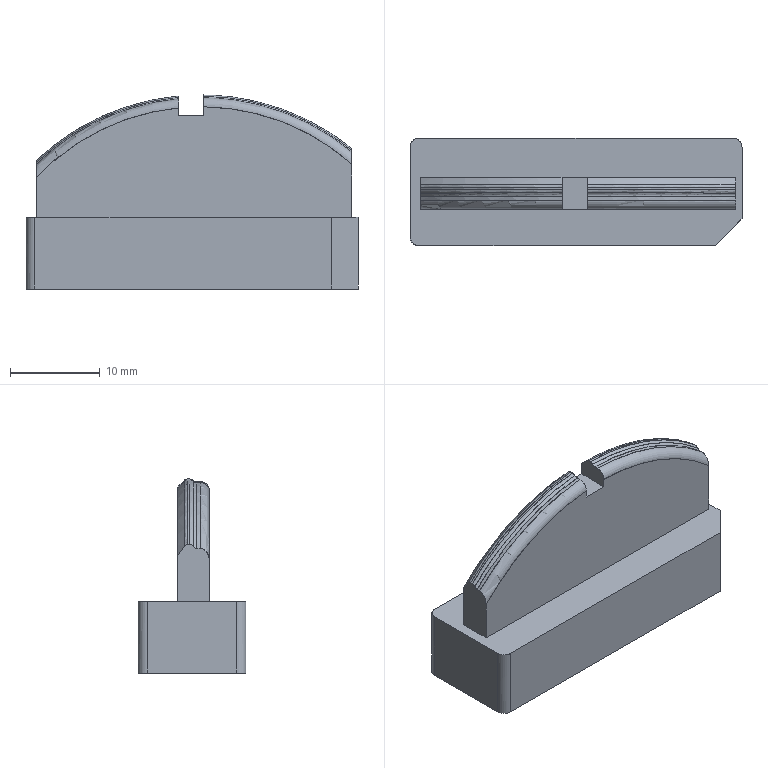NC program | PowerMill | posted with a generic post | part box 37 x 12 x 21.629 mm
Lines 4218 to 5227 of 105205:
N4315 M6
N4316 S18000 M03
N4317 G00 G90 X0.0 Y0.0
N4318 G43 Z9.7988 H2
N4319
N4320 G05 P10000 R4
N4321 X3.8878 Y-2.9665
N4322 Z0.7897
N4323 G01 Z-0.4103 F3600.0
N4324 X3.8963 Y-2.9462 F6000.0
N4325 G03 X3.7904 Y-2.687 I-0.1825 J0.0767
N4326 G01 X2.4727 Y-2.1337
N4327 X1.5291 Y-2.1962
N4328 X1.0573
N4329 X0.4881 Y-2.0472
N4330 X-0.0435 Y-1.7082
N4331 X-0.1285 Y-1.6385
N4332 X-0.2363 Y-1.6165
N4333 X-0.2982 Y-1.632
N4334 X-0.3524 Y-1.6656
N4335 X-0.4081 Y-1.7082
N4336 X-0.9761 Y-1.9746
N4337 X-1.4642 Y-2.0535
N4338 X-1.9522 Y-2.0109
N4339 X-2.4403 Y-1.9016
N4340 X-2.9283 Y-1.7353
N4341 X-3.4164 Y-1.4441
N4342 X-3.674 Y-1.2201
N4343 X-3.9044 Y-0.9501
N4344 X-4.0463 Y-0.7321
N4345 X-4.2366 Y-0.244
N4346 X-4.294 Y0.244
N4347 X-4.2782 Y0.7321
N4348 X-4.1535 Y1.2201
N4349 X-3.9044 Y1.6668
N4350 X-3.4164 Y2.1681
N4351 X-2.9283 Y2.4499
N4352 X-2.4403 Y2.6175
N4353 X-1.9522 Y2.7286
N4354 X-1.4642 Y2.7673
N4355 X-0.9721 Y2.6843
N4356 X-0.4881 Y2.4656
N4357 X-0.329 Y2.3453
N4358 G03 X-0.0873 Y2.3456 I0.1206 J0.1595
N4359 G01 X0.3915 Y2.6843
N4360 X0.9761 Y2.8772
N4361 X1.4642 Y2.8981
N4362 X2.9283 Y2.837
N4363 X4.1968 Y2.6843
N4364 X4.8805 Y2.4756
N4365 X5.3686 Y2.1934
N4366 X5.8566 Y1.7586
N4367 X6.1798 Y1.2201
N4368 X6.3053 Y0.7321
N4369 X6.3206 Y0.244
N4370 X6.2621 Y-0.244
N4371 X6.0746 Y-0.7321
N4372 X5.8566 Y-1.0433
N4373 X5.6918 Y-1.2201
N4374 X5.3686 Y-1.4742
N4375 X4.9939 Y-1.7082
N4376 X4.3925 Y-1.9103
N4377 X3.9044 Y-2.0193
N4378 X3.4164 Y-2.0712
N4379 X2.4727 Y-2.1337
N4380 X3.8379 Y-3.861 Z-0.6095
N4381 X3.845 Y-3.8401
N4382 G03 X3.7204 Y-3.5894 I-0.1877 J0.0631
N4383 G01 X2.6251 Y-3.221
N4384 X2.4403 Y-3.2469
N4385 X1.4642 Y-3.3354
N4386 X0.9761 Y-3.3249
N4387 X0.4881 Y-3.1909
N4388 X0.0 Y-2.8997
N4389 X-0.2247 Y-2.6843
N4390 X-0.4881 Y-2.3202
N4391 G03 X-0.7292 Y-2.2057 I-0.1848 J-0.0783
N4392 G01 X-0.7631 Y-2.2141
N4393 X-0.9761 Y-2.2972
N4394 X-1.4642 Y-2.373
N4395 X-1.9522 Y-2.3277
N4396 X-2.4086 Y-2.1962
N4397 X-3.4164 Y-2.0233
N4398 X-3.9044 Y-1.8926
N4399 X-4.3762 Y-1.7082
N4400 X-4.8805 Y-1.3566
N4401 X-5.0265 Y-1.2201
N4402 X-5.3938 Y-0.7321
N4403 X-5.5817 Y-0.244
N4404 X-5.6443 Y0.244
N4405 X-5.6293 Y0.7321
N4406 X-5.4997 Y1.2201
N4407 X-5.3686 Y1.4934
N4408 X-5.2253 Y1.7082
N4409 X-4.7414 Y2.1962
N4410 X-4.3925 Y2.4136
N4411 X-3.6666 Y2.6843
N4412 X-2.9283 Y2.8296
N4413 X-2.1966 Y2.9081
N4414 X-1.4642 Y2.9789
N4415 X-0.9761 Y2.8971
N4416 X-0.4881 Y2.6765
N4417 X-0.3206 Y2.5478
N4418 G03 X-0.0592 Y2.5632 I0.1218 J0.1586
N4419 G01 X0.0 Y2.6209
N4420 X0.4881 Y2.9295
N4421 X0.9761 Y3.0758
N4422 X1.4642 Y3.0975
N4423 X2.9283 Y3.0354
N4424 X4.8805 Y2.8382
N4425 X5.6708 Y2.6843
N4426 X6.3447 Y2.4334
N4427 X6.7366 Y2.1962
N4428 X7.1995 Y1.7082
N4429 X7.3208 Y1.5256
N4430 X7.4775 Y1.2201
N4431 X7.6024 Y0.7321
N4432 X7.618 Y0.244
N4433 X7.5605 Y-0.244
N4434 X7.3702 Y-0.7321
N4435 X7.0137 Y-1.2201
N4436 X6.8327 Y-1.4
N4437 X6.3662 Y-1.7082
N4438 X5.8566 Y-1.9131
N4439 X5.3686 Y-2.0345
N4440 X4.8561 Y-2.1286
N4441 X4.7929 Y-2.1517
N4442 X4.741 Y-2.1945
N4443 X4.6994 Y-2.2258
N4444 X4.3925 Y-2.5274
N4445 X3.9044 Y-2.8347
N4446 X3.4164 Y-3.0629
N4447 X2.9721 Y-3.1723
N4448 X2.6251 Y-3.221
N4449 X3.9626 Y-4.3928 Z-0.8087
N4450 X3.9715 Y-4.3727
N4451 G03 X3.87 Y-4.1117 I-0.1813 J0.0798
N4452 G01 X2.6422 Y-3.5712
N4453 X1.4642 Y-3.629
N4454 X0.9761 Y-3.6164
N4455 X0.4881 Y-3.482
N4456 X-0.0242 Y-3.1723
N4457 X-0.0726 Y-3.1264
N4458 X-0.1269 Y-3.0875
N4459 X-0.2342 Y-3.0664
N4460 X-0.3365 Y-3.1049
N4461 X-0.4277 Y-3.1723
N4462 X-0.9761 Y-3.4177
N4463 X-1.4642 Y-3.4877
N4464 X-1.9522 Y-3.4399
N4465 X-2.4403 Y-3.3415
N4466 X-2.9283 Y-3.2101
N4467 X-3.4164 Y-3.0341
N4468 X-3.9044 Y-2.7842
N4469 X-4.0276 Y-2.6843
N4470 X-4.3925 Y-2.2907
N4471 X-4.5536 Y-2.0708
N4472 X-4.6063 Y-2.0211
N4473 X-4.6731 Y-1.9931
N4474 X-4.8805 Y-1.9366
N4475 X-5.4041 Y-1.7082
N4476 X-5.8566 Y-1.4101
N4477 X-6.0488 Y-1.2201
N4478 X-6.3447 Y-0.8073
N4479 X-6.5793 Y-0.244
N4480 X-6.6352 Y0.244
N4481 X-6.6203 Y0.7321
N4482 X-6.4962 Y1.2201
N4483 X-6.2246 Y1.7082
N4484 X-5.8566 Y2.1269
N4485 X-5.3686 Y2.4407
N4486 X-4.8805 Y2.6524
N4487 X-4.3925 Y2.7842
N4488 X-3.4164 Y2.9556
N4489 X-1.9522 Y3.1436
N4490 X-1.4642 Y3.1767
N4491 X-0.9761 Y3.094
N4492 X-0.4881 Y2.8723
N4493 X-0.3213 Y2.7436
N4494 G03 X-0.0592 Y2.7591 I0.1222 J0.1584
N4495 G01 X0.0 Y2.8171
N4496 X0.4881 Y3.1271
N4497 X0.9761 Y3.2745
N4498 X1.4642 Y3.2968
N4499 X2.9283 Y3.2341
N4500 X4.8805 Y3.0355
N4501 X6.3447 Y2.7932
N4502 X6.8327 Y2.669
N4503 X7.3208 Y2.4661
N4504 X7.7708 Y2.1962
N4505 X8.2248 Y1.7082
N4506 X8.495 Y1.2201
N4507 X8.6159 Y0.7321
N4508 X8.6354 Y0.244
N4509 X8.5779 Y-0.244
N4510 X8.3836 Y-0.7321
N4511 X8.0455 Y-1.2201
N4512 X7.8088 Y-1.4489
N4513 X7.4022 Y-1.7082
N4514 X6.8327 Y-1.9529
N4515 X6.6666 Y-1.9979
N4516 X6.586 Y-2.0422
N4517 X6.5289 Y-2.1142
N4518 X5.9979 Y-2.6843
N4519 X5.8566 Y-2.7869
N4520 X5.3686 Y-3.0404
N4521 X5.0124 Y-3.1723
N4522 X4.3925 Y-3.3528
N4523 X3.9044 Y-3.4397
N4524 X2.9283 Y-3.5572
N4525 X2.6422 Y-3.5712
N4526 X4.0611 Y-4.6268 Z-1.008
N4527 X4.0702 Y-4.6068
N4528 G03 X3.9723 Y-4.3445 I-0.1801 J0.0822
N4529 G01 X2.6482 Y-3.7401
N4530 X1.4642 Y-3.7822
N4531 X0.9761 Y-3.7706
N4532 X0.5463 Y-3.6604
N4533 X0.0 Y-3.3497
N4534 X-0.0661 Y-3.292
N4535 X-0.1465 Y-3.2569
N4536 X-0.2343 Y-3.2599
N4537 X-0.3125 Y-3.2997
N4538 X-0.4881 Y-3.4277
N4539 X-0.9761 Y-3.6335
N4540 X-1.4642 Y-3.704
N4541 X-1.9522 Y-3.6695
N4542 X-2.9283 Y-3.551
N4543 X-3.9044 Y-3.3217
N4544 X-4.3392 Y-3.1723
N4545 X-4.8805 Y-2.9127
N4546 X-5.2132 Y-2.6843
N4547 X-5.3686 Y-2.5381
N4548 X-5.6407 Y-2.1962
N4549 X-5.7596 Y-1.9925
N4550 X-5.7973 Y-1.9457
N4551 X-5.8472 Y-1.9123
N4552 X-6.2807 Y-1.7082
N4553 X-6.8327 Y-1.3063
N4554 X-6.9162 Y-1.2201
N4555 X-7.238 Y-0.7321
N4556 X-7.4255 Y-0.244
N4557 X-7.4835 Y0.244
N4558 X-7.4686 Y0.7321
N4559 X-7.3422 Y1.2201
N4560 X-7.0895 Y1.7082
N4561 X-6.8327 Y2.0249
N4562 X-6.6406 Y2.1962
N4563 X-6.3447 Y2.3889
N4564 X-5.8566 Y2.6291
N4565 X-5.3686 Y2.7802
N4566 X-3.4164 Y3.1531
N4567 X-1.9522 Y3.3419
N4568 X-1.4642 Y3.3745
N4569 X-0.9761 Y3.2909
N4570 X-0.6766 Y3.1723
N4571 X-0.4881 Y3.068
N4572 X-0.3235 Y2.9405
N4573 G03 X-0.0762 Y2.9424 I0.1225 J0.1582
N4574 G01 X0.2117 Y3.1723
N4575 X0.4881 Y3.3248
N4576 X0.9761 Y3.4731
N4577 X1.4642 Y3.4962
N4578 X2.9283 Y3.4328
N4579 X4.8805 Y3.2329
N4580 X6.8327 Y2.8938
N4581 X7.8088 Y2.6505
N4582 X8.2969 Y2.426
N4583 X8.6492 Y2.1962
N4584 X8.7849 Y2.0809
N4585 X9.0988 Y1.7082
N4586 X9.3662 Y1.2201
N4587 X9.4911 Y0.7321
N4588 X9.5036 Y0.244
N4589 X9.4483 Y-0.244
N4590 X9.273 Y-0.703
N4591 X8.9252 Y-1.2201
N4592 X8.7849 Y-1.3628
N4593 X8.2969 Y-1.7083
N4594 X7.8336 Y-1.9224
N4595 X7.7919 Y-1.9482
N4596 X7.7578 Y-1.9835
N4597 X7.3208 Y-2.5628
N4598 X7.1924 Y-2.6843
N4599 X6.8327 Y-2.9249
N4600 X6.3404 Y-3.1723
N4601 X5.8566 Y-3.3369
N4602 X5.3686 Y-3.4671
N4603 X4.0422 Y-3.6604
N4604 X3.4164 Y-3.7129
N4605 X2.6482 Y-3.7401
N4606 X4.1087 Y-4.7676 Z-1.2072
N4607 X4.118 Y-4.7477
N4608 G03 X4.0223 Y-4.4846 I-0.1794 J0.0837
N4609 G01 X2.6511 Y-3.8449
N4610 X1.4642 Y-3.8771
N4611 X0.9761 Y-3.8605
N4612 X0.4881 Y-3.7299
N4613 X0.3383 Y-3.6604
N4614 X0.0 Y-3.4414
N4615 X-0.0817 Y-3.382
N4616 X-0.1813 Y-3.3652
N4617 X-0.234 Y-3.3774
N4618 X-0.2816 Y-3.4033
N4619 X-0.4881 Y-3.5555
N4620 X-0.6938 Y-3.6604
N4621 X-0.9761 Y-3.7606
N4622 X-1.4642 Y-3.8305
N4623 X-2.9283 Y-3.7299
N4624 X-4.3925 Y-3.5029
N4625 X-5.3617 Y-3.1723
N4626 X-5.8566 Y-2.8857
N4627 X-6.1444 Y-2.6843
N4628 X-6.3447 Y-2.4906
N4629 X-6.5634 Y-2.1962
N4630 X-6.7357 Y-1.9108
N4631 X-6.7674 Y-1.8709
N4632 X-6.8081 Y-1.8403
N4633 X-7.3208 Y-1.5488
N4634 X-7.6913 Y-1.2201
N4635 X-7.8088 Y-1.0692
N4636 X-8.009 Y-0.7321
N4637 X-8.1966 Y-0.244
N4638 X-8.2539 Y0.244
N4639 X-8.2387 Y0.7321
N4640 X-8.1137 Y1.2201
N4641 X-7.8661 Y1.7082
N4642 X-7.4173 Y2.1962
N4643 X-6.8327 Y2.5496
N4644 X-6.4673 Y2.6843
N4645 X-5.3686 Y2.9756
N4646 X-3.4164 Y3.3506
N4647 X-1.9522 Y3.5403
N4648 X-1.4642 Y3.5723
N4649 X-0.9761 Y3.4878
N4650 X-0.4881 Y3.2638
N4651 X-0.2702 Y3.0881
N4652 G03 X-0.0187 Y3.0904 I0.1244 J0.1517
N4653 G01 X-0.0091 Y3.0976
N4654 X0.0 Y3.1053
N4655 X0.4881 Y3.4175
N4656 X0.9761 Y3.5663
N4657 X1.4642 Y3.5944
N4658 X3.4164 Y3.5882
N4659 X4.8805 Y3.4302
N4660 X6.3447 Y3.1822
N4661 X8.2969 Y2.748
N4662 X8.7849 Y2.5668
N4663 X9.3984 Y2.1962
N4664 X9.7611 Y1.8311
N4665 X9.8495 Y1.7082
N4666 X10.1101 Y1.2201
N4667 X10.2329 Y0.7321
N4668 X10.2498 Y0.244
N4669 X10.191 Y-0.244
N4670 X10.0012 Y-0.7321
N4671 X9.6759 Y-1.2201
N4672 X9.273 Y-1.5722
N4673 X8.7788 Y-1.8484
N4674 X8.7334 Y-1.8831
N4675 X8.6997 Y-1.9293
N4676 X8.5583 Y-2.1962
N4677 X8.2969 Y-2.5317
N4678 X8.1355 Y-2.6843
N4679 X7.8088 Y-2.9139
N4680 X7.3718 Y-3.1723
N4681 X6.8327 Y-3.3737
N4682 X6.3447 Y-3.5075
N4683 X5.4876 Y-3.6604
N4684 X3.9044 Y-3.8109
N4685 X2.6511 Y-3.8449
N4686 X4.1434 Y-4.8695 Z-1.4065
N4687 X4.1529 Y-4.8497
N4688 G03 X4.0609 Y-4.5852 I-0.1782 J0.0862
N4689 G01 X2.6518 Y-3.9034
N4690 X1.4642 Y-3.9189
N4691 X0.9761 Y-3.9022
N4692 X0.4881 Y-3.7691
N4693 X0.2621 Y-3.6604
N4694 X-0.016 Y-3.4532
N4695 G03 X-0.2543 Y-3.4527 I-0.1195 J-0.1604
N4696 G01 X-0.4881 Y-3.6253
N4697 X-0.9761 Y-3.832
N4698 X-1.4642 Y-3.9014
N4699 X-2.9283 Y-3.8406
N4700 X-4.3925 Y-3.6927
N4701 X-5.3686 Y-3.4878
N4702 X-5.8566 Y-3.328
N4703 X-6.3447 Y-3.1144
N4704 X-6.9509 Y-2.6843
N4705 X-7.3208 Y-2.2739
N4706 X-7.5328 Y-1.8661
N4707 X-7.5658 Y-1.82
N4708 X-7.6105 Y-1.7851
N4709 X-7.744 Y-1.7082
N4710 X-8.2969 Y-1.2741
N4711 X-8.6746 Y-0.7321
N4712 X-8.7849 Y-0.4863
N4713 X-8.8594 Y-0.244
N4714 X-8.9203 Y0.244
N4715 X-8.9039 Y0.7321
N4716 X-8.7801 Y1.2201
N4717 X-8.5202 Y1.7082
N4718 X-8.2969 Y1.9906
N4719 X-8.0705 Y2.1962
N4720 X-7.8088 Y2.3807
N4721 X-7.3208 Y2.633
N4722 X-6.8327 Y2.7978
N4723 X-5.3481 Y3.1723
N4724 X-3.4164 Y3.5476
N4725 X-2.9283 Y3.5943
N4726 X-1.4642 Y3.5921
N4727 X-0.9761 Y3.5075
N4728 X-0.4881 Y3.2834
N4729 X-0.257 Y3.0956
N4730 X-0.2345 Y3.0821
N4731 G03 X0.0 Y3.1053 I0.1017 J0.1687
N4732 G01 X0.0226 Y3.1197
N4733 X0.0816 Y3.1723
N4734 X0.4881 Y3.4175
N4735 X0.9761 Y3.5663
N4736 X1.4642 Y3.5944
N4737 X4.8805 Y3.5943
N4738 X5.3686 Y3.5445
N4739 X6.3447 Y3.3787
N4740 X8.2969 Y2.9446
N4741 X9.1901 Y2.6843
N4742 X9.7611 Y2.4174
N4743 X10.0702 Y2.1962
N4744 X10.2491 Y2.0378
N4745 X10.5198 Y1.7082
N4746 X10.7372 Y1.2974
N4747 X10.8969 Y0.7321
N4748 X10.9129 Y0.244
N4749 X10.8549 Y-0.244
N4750 X10.6676 Y-0.7321
N4751 X10.3464 Y-1.2201
N4752 X10.2491 Y-1.3221
N4753 X9.7481 Y-1.7082
N4754 X9.6373 Y-1.773
N4755 X9.5936 Y-1.8074
N4756 X9.5612 Y-1.8526
N4757 X9.3805 Y-2.1962
N4758 X9.273 Y-2.3531
N4759 X8.9625 Y-2.6843
N4760 X8.2969 Y-3.1458
N4761 X7.3208 Y-3.4985
N4762 X6.5944 Y-3.6604
N4763 X5.3686 Y-3.8089
N4764 X3.9044 Y-3.8871
N4765 X2.6518 Y-3.9034
N4766 X4.1108 Y-4.882 Z-1.6057
N4767 X4.1205 Y-4.8622
N4768 G03 X4.03 Y-4.5973 I-0.1777 J0.0872
N4769 G01 X2.652 Y-3.9208
N4770 X1.4642 Y-3.9295
N4771 X0.9761 Y-3.9109
N4772 X0.4881 Y-3.7792
N4773 X0.2467 Y-3.6604
N4774 X-0.0063 Y-3.4716
N4775 G03 X-0.2451 Y-3.4712 I-0.1196 J-0.1602
N4776 G01 X-0.5001 Y-3.6604
N4777 X-0.9761 Y-3.8577
N4778 X-1.4642 Y-3.9266
N4779 X-2.9283 Y-3.9031
N4780 X-4.3925 Y-3.8143
N4781 X-5.3686 Y-3.683
N4782 X-6.3447 Y-3.4337
N4783 X-6.8327 Y-3.2345
N4784 X-7.3208 Y-2.9655
N4785 X-7.8088 Y-2.5778
N4786 X-8.115 Y-2.1962
N4787 X-8.2974 Y-1.803
N4788 X-8.3238 Y-1.7607
N4789 X-8.3598 Y-1.7264
N4790 X-8.7849 Y-1.4117
N4791 X-8.9773 Y-1.2201
N4792 X-9.273 Y-0.7696
N4793 X-9.47 Y-0.244
N4794 X-9.5277 Y0.244
N4795 X-9.5087 Y0.7321
N4796 X-9.3865 Y1.2201
N4797 X-9.273 Y1.4906
N4798 X-9.1502 Y1.7082
N4799 X-8.7849 Y2.1257
N4800 X-8.2969 Y2.4844
N4801 X-7.8381 Y2.6843
N4802 X-6.8327 Y2.9905
N4803 X-5.3686 Y3.3613
N4804 X-4.3925 Y3.5611
N4805 X-3.9044 Y3.5943
N4806 X-2.937 Y3.5935
N4807 X-2.9283 Y3.5943
N4808 X-1.5709 Y3.5922
N4809 X-1.4642 Y3.5921
N4810 X-0.9761 Y3.5075
N4811 X-0.4881 Y3.2834
N4812 X-0.257 Y3.0957
N4813 X-0.2344 Y3.082
N4814 G03 X0.0001 Y3.1053 I0.1017 J0.1688
N4815 G01 X0.0224 Y3.1195
N4816 X0.0816 Y3.1723
N4817 X0.4881 Y3.4175
N4818 X0.9761 Y3.5663
N4819 X1.4642 Y3.5944
N4820 X5.8566 Y3.5943
N4821 X6.3447 Y3.5738
N4822 X8.2969 Y3.137
N4823 X9.7611 Y2.7124
N4824 X10.2491 Y2.5033
N4825 X10.7044 Y2.1962
N4826 X11.1537 Y1.7082
N4827 X11.3983 Y1.2201
N4828 X11.5225 Y0.7321
N4829 X11.5387 Y0.244
N4830 X11.4806 Y-0.244
N4831 X11.2986 Y-0.7321
N4832 X10.9805 Y-1.2201
N4833 X10.7372 Y-1.4548
N4834 X10.3526 Y-1.7241
N4835 X10.3153 Y-1.7579
N4836 X10.2877 Y-1.8
N4837 X10.0937 Y-2.1962
N4838 X9.7611 Y-2.6066
N4839 X9.273 Y-2.9929
N4840 X8.9677 Y-3.1723
N4841 X8.2969 Y-3.4514
N4842 X7.4686 Y-3.6604
N4843 X6.3447 Y-3.8217
N4844 X4.8805 Y-3.9045
N4845 X2.652 Y-3.9208
N4846 X4.0798 Y-4.8888 Z-1.805
N4847 X4.0897 Y-4.8691
N4848 G03 X4.0011 Y-4.6035 I-0.1771 J0.0885
N4849 G01 X2.652 Y-3.9293
N4850 X1.4642 Y-3.9295
N4851 X0.9761 Y-3.9109
N4852 X0.4881 Y-3.7792
N4853 X0.2467 Y-3.6604
N4854 X-0.0045 Y-3.4731
N4855 G03 X-0.2434 Y-3.473 I-0.1196 J-0.1603
N4856 G01 X-0.4954 Y-3.6604
N4857 X-0.9761 Y-3.8611
N4858 X-1.4642 Y-3.928
N4859 X-3.9044 Y-3.9079
N4860 X-5.3686 Y-3.8072
N4861 X-6.2427 Y-3.6604
N4862 X-6.8327 Y-3.5089
N4863 X-7.3208 Y-3.329
N4864 X-7.8088 Y-3.0817
N4865 X-8.3186 Y-2.6843
N4866 X-8.7389 Y-2.1962
N4867 X-8.9494 Y-1.7465
N4868 X-8.9752 Y-1.7053
N4869 X-9.0102 Y-1.6715
N4870 X-9.273 Y-1.4736
N4871 X-9.5398 Y-1.2201
N4872 X-9.7611 Y-0.9108
N4873 X-9.8538 Y-0.7321
N4874 X-10.034 Y-0.244
N4875 X-10.0922 Y0.244
N4876 X-10.0751 Y0.7321
N4877 X-9.9515 Y1.2201
N4878 X-9.7125 Y1.7082
N4879 X-9.273 Y2.1875
N4880 X-8.7849 Y2.5242
N4881 X-8.4253 Y2.6843
N4882 X-6.8327 Y3.1831
N4883 X-5.3686 Y3.5519
N4884 X-4.8805 Y3.5943
N4885 X-3.9129 Y3.5937
N4886 X-3.9044 Y3.5943
N4887 X-2.937 Y3.5934
N4888 X-2.9283 Y3.5942
N4889 X-1.6139 Y3.5922
N4890 X-1.4642 Y3.5921
N4891 X-0.9761 Y3.5075
N4892 X-0.4881 Y3.2835
N4893 X-0.257 Y3.0957
N4894 X-0.2343 Y3.082
N4895 G03 X0.0001 Y3.1052 I0.1016 J0.1688
N4896 G01 X0.0221 Y3.1193
N4897 X0.0815 Y3.1723
N4898 X0.4881 Y3.4175
N4899 X0.9761 Y3.5663
N4900 X1.4642 Y3.5944
N4901 X6.8327 Y3.5943
N4902 X7.3208 Y3.5604
N4903 X8.2969 Y3.3294
N4904 X10.2491 Y2.7537
N4905 X10.7372 Y2.548
N4906 X11.2252 Y2.2251
N4907 X11.7133 Y1.7007
N4908 X11.9463 Y1.2201
N4909 X12.0712 Y0.7321
N4910 X12.0864 Y0.244
N4911 X12.0291 Y-0.244
N4912 X11.853 Y-0.7321
N4913 X11.7133 Y-0.9849
N4914 X11.5382 Y-1.2201
N4915 X11.2252 Y-1.5099
N4916 X11.0207 Y-1.6655
N4917 X10.9867 Y-1.6984
N4918 X10.9614 Y-1.7383
N4919 X10.7422 Y-2.1962
N4920 X10.3212 Y-2.6843
N4921 X9.7611 Y-3.1155
N4922 X9.273 Y-3.3493
N4923 X8.7849 Y-3.517
N4924 X8.2435 Y-3.6604
N4925 X7.3208 Y-3.8104
N4926 X6.3447 Y-3.8908
N4927 X4.8805 Y-3.9288
N4928 X2.652 Y-3.9293
N4929 X4.0839 Y-4.8914 Z-2.0043
N4930 X4.0937 Y-4.8718
N4931 G03 X4.0052 Y-4.6061 I-0.1771 J0.0886
N4932 G01 X2.652 Y-3.9295
N4933 X1.4642
N4934 X0.9761 Y-3.9109
N4935 X0.4881 Y-3.7792
N4936 X0.2467 Y-3.6604
N4937 X-0.0045 Y-3.4731
N4938 G03 X-0.2434 Y-3.473 I-0.1195 J-0.1604
N4939 G01 X-0.4954 Y-3.6604
N4940 X-0.9761 Y-3.8642
N4941 X-1.4642 Y-3.9284
N4942 X-3.9044 Y-3.9295
N4943 X-4.8805 Y-3.9062
N4944 X-5.8566 Y-3.8343
N4945 X-6.8327 Y-3.6844
N4946 X-7.8088 Y-3.3908
N4947 X-8.2969 Y-3.1573
N4948 X-8.7849 Y-2.8196
N4949 X-8.9412 Y-2.6843
N4950 X-9.273 Y-2.3158
N4951 X-9.3528 Y-2.1962
N4952 X-9.5666 Y-1.7056
N4953 X-9.5879 Y-1.6682
N4954 X-9.6167 Y-1.6363
N4955 X-10.0824 Y-1.2201
N4956 X-10.2491 Y-1.0013
N4957 X-10.3976 Y-0.7321
N4958 X-10.5667 Y-0.244
N4959 X-10.6262 Y0.244
N4960 X-10.6084 Y0.7321
N4961 X-10.4877 Y1.2201
N4962 X-10.2553 Y1.7082
N4963 X-9.8122 Y2.1962
N4964 X-9.273 Y2.5577
N4965 X-8.9964 Y2.6843
N4966 X-6.8327 Y3.3757
N4967 X-6.3447 Y3.503
N4968 X-5.8566 Y3.5905
N4969 X-5.3686 Y3.5944
N4970 X-4.8899 Y3.5941
N4971 X-4.8852
N4972 X-4.8805 Y3.5943
N4973 X-3.9129 Y3.5937
N4974 X-3.9044 Y3.5942
N4975 X-2.9465 Y3.5934
N4976 X-2.9374 Y3.5936
N4977 X-2.9283 Y3.5942
N4978 X-1.6689 Y3.5923
N4979 X-1.4642 Y3.5921
N4980 X-0.9761 Y3.5075
N4981 X-0.4881 Y3.2835
N4982 X-0.257 Y3.0957
N4983 X-0.2341 Y3.0819
N4984 G03 X0.0001 Y3.1052 I0.1015 J0.1688
N4985 G01 X0.0219 Y3.1191
N4986 X0.0815 Y3.1723
N4987 X0.4881 Y3.4175
N4988 X0.9761 Y3.5663
N4989 X1.4642 Y3.5944
N4990 X1.6781 Y3.5943
N4991 X6.8327
N4992 X6.8507 Y3.5931
N4993 X7.8088 Y3.5928
N4994 X8.2969 Y3.5218
N4995 X9.7611 Y3.0922
N4996 X10.9796 Y2.6843
N4997 X11.2252 Y2.5742
N4998 X11.7133 Y2.2731
N4999 X12.2013 Y1.7902
N5000 X12.494 Y1.2201
N5001 X12.6188 Y0.7321
N5002 X12.6341 Y0.244
N5003 X12.5768 Y-0.244
N5004 X12.4006 Y-0.7321
N5005 X12.2013 Y-1.0696
N5006 X12.0859 Y-1.2201
N5007 X11.6207 Y-1.6261
N5008 X11.5916 Y-1.6576
N5009 X11.5699 Y-1.6946
N5010 X11.3438 Y-2.1962
N5011 X11.2252 Y-2.3686
N5012 X10.7372 Y-2.8505
N5013 X10.2556 Y-3.1723
N5014 X9.7611 Y-3.4118
N5015 X8.9557 Y-3.6604
N5016 X8.2969 Y-3.7754
N5017 X7.3208 Y-3.8828
N5018 X5.8566 Y-3.9295
N5019 X2.652
N5020 X4.0856 Y-4.8923 Z-2.2035
N5021 X4.0954 Y-4.8726
N5022 G03 X4.0069 Y-4.607 I-0.1771 J0.0885
N5023 G01 X2.652 Y-3.9295
N5024 X1.4642
N5025 X0.9761 Y-3.9109
N5026 X0.4881 Y-3.7793
N5027 X0.2467 Y-3.6604
N5028 X-0.0041 Y-3.4734
N5029 G03 X-0.2441 Y-3.474 I-0.1196 J-0.1603
N5030 G01 X-0.4881 Y-3.6579
N5031 X-0.9761 Y-3.8673
N5032 X-1.4642 Y-3.9288
N5033 X-3.2447 Y-3.9292
N5034 X-3.9044 Y-3.9295
N5035 X-3.911 Y-3.9293
N5036 X-4.8805 Y-3.9295
N5037 X-5.8566 Y-3.8997
N5038 X-6.8327 Y-3.8027
N5039 X-7.5746 Y-3.6604
N5040 X-8.2969 Y-3.4385
N5041 X-8.8332 Y-3.1723
N5042 X-9.273 Y-2.8798
N5043 X-9.7611 Y-2.3794
N5044 X-9.8875 Y-2.1962
N5045 X-10.1334 Y-1.6481
N5046 X-10.1536 Y-1.6131
N5047 X-10.1804 Y-1.5828
N5048 X-10.5744 Y-1.2201
N5049 X-10.7372 Y-1.0027
N5050 X-10.889 Y-0.7321
N5051 X-11.0596 Y-0.244
N5052 X-11.1175 Y0.244
N5053 X-11.101 Y0.7321
N5054 X-10.9795 Y1.2201
N5055 X-10.7465 Y1.7082
N5056 X-10.3048 Y2.1962
N5057 X-9.7611 Y2.5606
N5058 X-9.5038 Y2.6843
N5059 X-8.7849 Y2.9492
N5060 X-6.8327 Y3.5559
N5061 X-6.3447 Y3.5943
N5062 X-5.4149 Y3.5939
N5063 X-5.3686 Y3.5943
N5064 X-4.8831 Y3.594
N5065 X-4.8805 Y3.5942
N5066 X-3.9129 Y3.5936
N5067 X-3.9044 Y3.5942
N5068 X-2.937 Y3.5933
N5069 X-2.9283 Y3.5941
N5070 X-1.708 Y3.5923
N5071 X-1.4642 Y3.5922
N5072 X-0.9761 Y3.5075
N5073 X-0.4881 Y3.2835
N5074 X-0.257 Y3.0957
N5075 X-0.234 Y3.0819
N5076 G03 X0.0002 Y3.1051 I0.1014 J0.1688
N5077 G01 X0.0216 Y3.1189
N5078 X0.0815 Y3.1723
N5079 X0.4881 Y3.4175
N5080 X0.9761 Y3.5663
N5081 X1.4642 Y3.5944
N5082 X8.2969 Y3.5943
N5083 X8.7849 Y3.5632
N5084 X9.7611 Y3.2827
N5085 X11.5161 Y2.6843
N5086 X11.7133 Y2.5902
N5087 X12.2013 Y2.2883
N5088 X12.6894 Y1.7907
N5089 X12.9827 Y1.2201
N5090 X13.1073 Y0.7321
N5091 X13.1225 Y0.244
N5092 X13.0652 Y-0.244
N5093 X12.8891 Y-0.7321
N5094 X12.6894 Y-1.0735
N5095 X12.5735 Y-1.2201
N5096 X12.1694 Y-1.5936
N5097 X12.1417 Y-1.6251
N5098 X12.1213 Y-1.6617
N5099 X11.8921 Y-2.1962
N5100 X11.7133 Y-2.4398
N5101 X11.2252 Y-2.9264
N5102 X10.8456 Y-3.1723
N5103 X10.2491 Y-3.453
N5104 X9.571 Y-3.6604
N5105 X8.7849 Y-3.8124
N5106 X7.8088 Y-3.9015
N5107 X6.8327 Y-3.9295
N5108 X2.652
N5109 X4.0795 Y-4.8893 Z-2.4028
N5110 X4.0894 Y-4.8696
N5111 G03 X4.0008 Y-4.6039 I-0.1771 J0.0886
N5112 G01 X2.652 Y-3.9295
N5113 X1.4642
N5114 X0.9761 Y-3.911
N5115 X0.4881 Y-3.7793
N5116 X0.2466 Y-3.6604
N5117 X-0.0045 Y-3.4731
N5118 G03 X-0.2441 Y-3.4739 I-0.1193 J-0.1603
N5119 G01 X-0.4881 Y-3.6578
N5120 X-0.5692 Y-3.6926
N5121 X-0.9761 Y-3.8704
N5122 X-1.4642 Y-3.9292
N5123 X-3.8177 Y-3.9294
N5124 X-3.9044
N5125 X-3.9062
N5126 X-3.9079
N5127 X-5.3686 Y-3.9295
N5128 X-6.3447 Y-3.9082
N5129 X-7.3208 Y-3.8207
N5130 X-8.1568 Y-3.6604
N5131 X-8.7849 Y-3.4547
N5132 X-9.273 Y-3.2234
N5133 X-9.7611 Y-2.9173
N5134 X-10.2491 Y-2.4342
N5135 X-10.4222 Y-2.1962
N5136 X-10.6631 Y-1.6201
N5137 X-10.6833 Y-1.5833
N5138 X-10.7107 Y-1.5515
N5139 X-11.0634 Y-1.2201
N5140 X-11.2252 Y-1.0073
N5141 X-11.3789 Y-0.7321
N5142 X-11.5467 Y-0.244
N5143 X-11.6046 Y0.244
N5144 X-11.5892 Y0.7321
N5145 X-11.4662 Y1.2201
N5146 X-11.2363 Y1.7082
N5147 X-10.7975 Y2.1962
N5148 X-10.2491 Y2.5623
N5149 X-9.9953 Y2.6843
N5150 X-8.2969 Y3.2984
N5151 X-7.3208 Y3.5773
N5152 X-6.8367 Y3.5943
N5153 X-6.3523 Y3.5942
N5154 X-6.3485
N5155 X-6.3447 Y3.5943
N5156 X-5.4149 Y3.5939
N5157 X-5.3686 Y3.5943
N5158 X-4.8899 Y3.594
N5159 X-4.8852
N5160 X-4.8805 Y3.5942
N5161 X-3.9129 Y3.5936
N5162 X-3.9044 Y3.5941
N5163 X-2.9465 Y3.5933
N5164 X-2.9374 Y3.5935
N5165 X-2.9283 Y3.5941
N5166 X-1.7571 Y3.5923
N5167 X-1.4642 Y3.5922
N5168 X-0.9761 Y3.5076
N5169 X-0.4881 Y3.2835
N5170 X-0.257 Y3.0957
N5171 X-0.2339 Y3.0818
N5172 G03 X0.0002 Y3.1051 I0.1014 J0.1689
N5173 G01 X0.0214 Y3.1186
N5174 X0.0815 Y3.1723
N5175 X0.4881 Y3.4176
N5176 X0.9761 Y3.5664
N5177 X1.4642 Y3.5944
N5178 X8.7849
N5179 X9.273 Y3.583
N5180 X9.7611 Y3.4733
N5181 X12.0028 Y2.6843
N5182 X12.6894 Y2.2827
N5183 X13.1774 Y1.7795
N5184 X13.4588 Y1.2201
N5185 X13.5828 Y0.7321
N5186 X13.5981 Y0.244
N5187 X13.5407 Y-0.244
N5188 X13.3674 Y-0.7321
N5189 X13.1774 Y-1.0643
N5190 X13.0531 Y-1.2201
N5191 X12.7099 Y-1.5447
N5192 X12.6836 Y-1.5752
N5193 X12.6639 Y-1.6103
N5194 X12.4096 Y-2.1962
N5195 X12.2013 Y-2.475
N5196 X11.7133 Y-2.9494
N5197 X11.3637 Y-3.1723
N5198 X10.7372 Y-3.473
N5199 X10.1726 Y-3.6604
N5200 X9.273 Y-3.8259
N5201 X8.7849 Y-3.8788
N5202 X7.3208 Y-3.9295
N5203 X2.652
N5204 X4.0908 Y-4.8949 Z-2.602
N5205 X4.1007 Y-4.8752
N5206 G03 X4.0121 Y-4.6096 I-0.1771 J0.0885
N5207 G01 X2.652 Y-3.9295
N5208 X-6.3447
N5209 X-6.8327 Y-3.9134
N5210 X-7.8088 Y-3.8325
N5211 X-8.6928 Y-3.6604
N5212 X-9.273 Y-3.4708
N5213 X-9.7611 Y-3.2472
N5214 X-10.2491 Y-2.9256
N5215 X-10.5007 Y-2.6843
N5216 X-10.7372 Y-2.4149
N5217 X-10.894 Y-2.1962
N5218 X-11.11 Y-1.7082
N5219 X-11.1296 Y-1.6339
N5220 X-11.1586 Y-1.5627
N5221 X-11.1904 Y-1.5222
N5222 X-11.1995 Y-1.5132
N5223 X-11.4986 Y-1.2201
N5224 X-11.7133 Y-0.9194
N5225 X-11.8138 Y-0.7321
N5226 X-11.9951 Y-0.244
N5227 X-12.05 Y0.244
N5228 X-12.0372 Y0.7321
N5229 X-11.9099 Y1.2201
N5230 X-11.7133 Y1.6389
N5231 X-11.2428 Y2.1962
N5232 X-10.7372 Y2.5483
N5233 X-10.4678 Y2.6843
N5234 X-8.2969 Y3.4877
N5235 X-7.8088 Y3.588
N5236 X-7.3208 Y3.5944
N5237 X8.7849
N5238 X9.7611 Y3.5905
N5239 X10.2491 Y3.4972
N5240 X11.7133 Y2.9821
N5241 X12.203 Y2.7828
N5242 X12.6894 Y2.5754
N5243 X13.1774 Y2.2598
N5244 X13.6757 Y1.7082
N5245 X13.9118 Y1.2201
N5246 X14.0335 Y0.7321
N5247 X14.0497 Y0.244
N5248 X13.9903 Y-0.244
N5249 X13.8184 Y-0.7321
N5250 X13.6655 Y-1.0061
N5251 X13.5032 Y-1.2201
N5252 X13.1978 Y-1.5214
N5253 X13.1661 Y-1.5621
N5254 X13.1458 Y-1.6096
N5255 X13.1181 Y-1.7082
N5256 X12.9014 Y-2.1962
N5257 X12.5152 Y-2.6843
N5258 X12.2013 Y-2.9723
N5259 X11.8811 Y-3.1723
N5260 X11.2252 Y-3.4836
N5261 X10.6907 Y-3.6604
N5262 X10.2491 Y-3.7605
N5263 X9.273 Y-3.8911
N5264 X8.2969 Y-3.9295
N5265 X2.652
N5266 X4.0908 Y-4.8949 Z-2.8012
N5267 X4.1007 Y-4.8752
N5268 G03 X4.0121 Y-4.6096 I-0.1771 J0.0885
N5269 G01 X2.652 Y-3.9295
N5270 X-6.8327
N5271 X-7.8088 Y-3.8962
N5272 X-8.7849 Y-3.7579
N5273 X-9.273 Y-3.6442
N5274 X-9.7611 Y-3.4671
N5275 X-10.2491 Y-3.233
N5276 X-10.7372 Y-2.9061
N5277 X-10.9672 Y-2.6843
N5278 X-11.3597 Y-2.1962
N5279 X-11.5753 Y-1.7082
N5280 X-11.6136 Y-1.5742
N5281 X-11.6272 Y-1.5386
N5282 X-11.6492 Y-1.5076
N5283 X-11.6649 Y-1.4874
N5284 X-11.9338 Y-1.2201
N5285 X-12.2013 Y-0.8268
N5286 X-12.4189 Y-0.244
N5287 X-12.4759 Y0.244
N5288 X-12.4612 Y0.7321
N5289 X-12.3377 Y1.2201
N5290 X-12.2013 Y1.5455
N5291 X-12.1063 Y1.7082
N5292 X-11.7133 Y2.1617
N5293 X-11.2252 Y2.5178
N5294 X-10.9098 Y2.6843
N5295 X-10.2491 Y2.955
N5296 X-8.7849 Y3.4993
N5297 X-8.2969 Y3.5901
N5298 X-7.8088 Y3.5944
N5299 X-6.9711 Y3.5943
N5300 X8.7849
N5301 X9.0261 Y3.5933
N5302 X10.2491
N5303 X10.7372 Y3.5176
N5304 X11.6972 Y3.1723
N5305 X12.9077 Y2.6843
N5306 X13.1774 Y2.5465
N5307 X13.6655 Y2.2032
N5308 X14.0998 Y1.7082
N5309 X14.3362 Y1.2201
N5310 X14.4611 Y0.7321
N5311 X14.4756 Y0.244
N5312 X14.4188 Y-0.244
N5313 X14.2427 Y-0.7321
N5314 X14.1535 Y-0.9014
N5315 X13.9266 Y-1.2201
N5316 X13.6576 Y-1.4902
N5317 X13.6266 Y-1.5305
N5318 X13.6067 Y-1.5773
N5319 X13.57 Y-1.7082
N5320 X13.3529 Y-2.1962
N5321 X12.9663 Y-2.6843
N5322 X12.6894 Y-2.9448
N5323 X12.2013 Y-3.2665
N5324 X11.7133 Y-3.4906